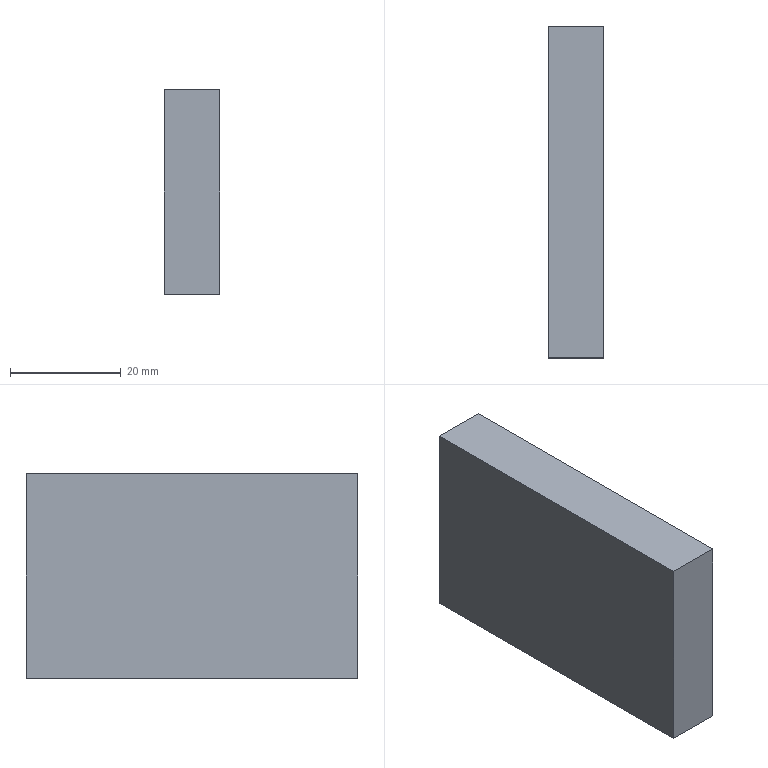Part | NX | features DATUM_CSYS 2, EXTRUDE 1, SKETCH 1 | 1 solid | 6 faces | box 10 x 60 x 37 mm | volume 22200 mm3 | plane 6
STEP:
#1=CARTESIAN_POINT('',(0.,-30.,18.5));
#2=VERTEX_POINT('',#1);
#3=CARTESIAN_POINT('',(0.,-30.,-18.5));
#4=VERTEX_POINT('',#3);
#5=CARTESIAN_POINT('',(0.,-30.,18.5));
#6=DIRECTION('',(0.,0.,-1.));
#7=VECTOR('',#6,1000.);
#8=LINE('',#5,#7);
#9=EDGE_CURVE('',#2,#4,#8,.T.);
#10=ORIENTED_EDGE('',*,*,#9,.T.);
#11=CARTESIAN_POINT('',(10.,-30.,-18.5));
#12=VERTEX_POINT('',#11);
#13=CARTESIAN_POINT('',(10.,-30.,-18.5));
#14=DIRECTION('',(-1.,0.,0.));
#15=VECTOR('',#14,1000.);
#16=LINE('',#13,#15);
#17=EDGE_CURVE('',#12,#4,#16,.T.);
#18=ORIENTED_EDGE('',*,*,#17,.F.);
#19=CARTESIAN_POINT('',(10.,-30.,18.5));
#20=VERTEX_POINT('',#19);
#21=CARTESIAN_POINT('',(10.,-30.,18.5));
#22=DIRECTION('',(0.,0.,-1.));
#23=VECTOR('',#22,1000.);
#24=LINE('',#21,#23);
#25=EDGE_CURVE('',#20,#12,#24,.T.);
#26=ORIENTED_EDGE('',*,*,#25,.F.);
#27=CARTESIAN_POINT('',(10.,-30.,18.5));
#28=DIRECTION('',(-1.,0.,0.));
#29=VECTOR('',#28,1000.);
#30=LINE('',#27,#29);
#31=EDGE_CURVE('',#20,#2,#30,.T.);
#32=ORIENTED_EDGE('',*,*,#31,.T.);
#33=EDGE_LOOP('',(#10,#18,#26,#32));
#34=FACE_BOUND('',#33,.T.);
#35=CARTESIAN_POINT('',(10.,-30.,18.5));
#36=DIRECTION('',(0.,1.,0.));
#37=DIRECTION('',(0.,0.,1.));
#38=AXIS2_PLACEMENT_3D('',#35,#36,#37);
#39=PLANE('',#38);
#40=ADVANCED_FACE('',(#34),#39,.F.);
#41=CARTESIAN_POINT('',(0.,30.,-18.5));
#42=VERTEX_POINT('',#41);
#43=CARTESIAN_POINT('',(0.,-30.,-18.5));
#44=DIRECTION('',(0.,1.,0.));
#45=VECTOR('',#44,1000.);
#46=LINE('',#43,#45);
#47=EDGE_CURVE('',#4,#42,#46,.T.);
#48=ORIENTED_EDGE('',*,*,#47,.T.);
#49=CARTESIAN_POINT('',(10.,30.,-18.5));
#50=VERTEX_POINT('',#49);
#51=CARTESIAN_POINT('',(10.,30.,-18.5));
#52=DIRECTION('',(-1.,0.,0.));
#53=VECTOR('',#52,1000.);
#54=LINE('',#51,#53);
#55=EDGE_CURVE('',#50,#42,#54,.T.);
#56=ORIENTED_EDGE('',*,*,#55,.F.);
#57=CARTESIAN_POINT('',(10.,-30.,-18.5));
#58=DIRECTION('',(0.,1.,0.));
#59=VECTOR('',#58,1000.);
#60=LINE('',#57,#59);
#61=EDGE_CURVE('',#12,#50,#60,.T.);
#62=ORIENTED_EDGE('',*,*,#61,.F.);
#63=ORIENTED_EDGE('',*,*,#17,.T.);
#64=EDGE_LOOP('',(#48,#56,#62,#63));
#65=FACE_BOUND('',#64,.T.);
#66=CARTESIAN_POINT('',(10.,-30.,-18.5));
#67=DIRECTION('',(0.,0.,1.));
#68=DIRECTION('',(1.,0.,0.));
#69=AXIS2_PLACEMENT_3D('',#66,#67,#68);
#70=PLANE('',#69);
#71=ADVANCED_FACE('',(#65),#70,.F.);
#72=CARTESIAN_POINT('',(0.,30.,18.5));
#73=VERTEX_POINT('',#72);
#74=CARTESIAN_POINT('',(0.,30.,-18.5));
#75=DIRECTION('',(0.,0.,1.));
#76=VECTOR('',#75,1000.);
#77=LINE('',#74,#76);
#78=EDGE_CURVE('',#42,#73,#77,.T.);
#79=ORIENTED_EDGE('',*,*,#78,.T.);
#80=CARTESIAN_POINT('',(10.,30.,18.5));
#81=VERTEX_POINT('',#80);
#82=CARTESIAN_POINT('',(10.,30.,18.5));
#83=DIRECTION('',(-1.,0.,0.));
#84=VECTOR('',#83,1000.);
#85=LINE('',#82,#84);
#86=EDGE_CURVE('',#81,#73,#85,.T.);
#87=ORIENTED_EDGE('',*,*,#86,.F.);
#88=CARTESIAN_POINT('',(10.,30.,-18.5));
#89=DIRECTION('',(0.,0.,1.));
#90=VECTOR('',#89,1000.);
#91=LINE('',#88,#90);
#92=EDGE_CURVE('',#50,#81,#91,.T.);
#93=ORIENTED_EDGE('',*,*,#92,.F.);
#94=ORIENTED_EDGE('',*,*,#55,.T.);
#95=EDGE_LOOP('',(#79,#87,#93,#94));
#96=FACE_BOUND('',#95,.T.);
#97=CARTESIAN_POINT('',(10.,30.,-18.5));
#98=DIRECTION('',(0.,-1.,0.));
#99=DIRECTION('',(0.,0.,-1.));
#100=AXIS2_PLACEMENT_3D('',#97,#98,#99);
#101=PLANE('',#100);
#102=ADVANCED_FACE('',(#96),#101,.F.);
#103=CARTESIAN_POINT('',(0.,30.,18.5));
#104=DIRECTION('',(0.,-1.,0.));
#105=VECTOR('',#104,1000.);
#106=LINE('',#103,#105);
#107=EDGE_CURVE('',#73,#2,#106,.T.);
#108=ORIENTED_EDGE('',*,*,#107,.T.);
#109=ORIENTED_EDGE('',*,*,#31,.F.);
#110=CARTESIAN_POINT('',(10.,30.,18.5));
#111=DIRECTION('',(0.,-1.,0.));
#112=VECTOR('',#111,1000.);
#113=LINE('',#110,#112);
#114=EDGE_CURVE('',#81,#20,#113,.T.);
#115=ORIENTED_EDGE('',*,*,#114,.F.);
#116=ORIENTED_EDGE('',*,*,#86,.T.);
#117=EDGE_LOOP('',(#108,#109,#115,#116));
#118=FACE_BOUND('',#117,.T.);
#119=CARTESIAN_POINT('',(10.,30.,18.5));
#120=DIRECTION('',(0.,0.,-1.));
#121=DIRECTION('',(-1.,0.,0.));
#122=AXIS2_PLACEMENT_3D('',#119,#120,#121);
#123=PLANE('',#122);
#124=ADVANCED_FACE('',(#118),#123,.F.);
#125=ORIENTED_EDGE('',*,*,#25,.T.);
#126=ORIENTED_EDGE('',*,*,#61,.T.);
#127=ORIENTED_EDGE('',*,*,#92,.T.);
#128=ORIENTED_EDGE('',*,*,#114,.T.);
#129=EDGE_LOOP('',(#125,#126,#127,#128));
#130=FACE_BOUND('',#129,.T.);
#131=CARTESIAN_POINT('',(10.,0.,0.));
#132=DIRECTION('',(1.,0.,0.));
#133=DIRECTION('',(0.,0.,-1.));
#134=AXIS2_PLACEMENT_3D('',#131,#132,#133);
#135=PLANE('',#134);
#136=ADVANCED_FACE('',(#130),#135,.T.);
#137=ORIENTED_EDGE('',*,*,#9,.F.);
#138=ORIENTED_EDGE('',*,*,#107,.F.);
#139=ORIENTED_EDGE('',*,*,#78,.F.);
#140=ORIENTED_EDGE('',*,*,#47,.F.);
#141=EDGE_LOOP('',(#137,#138,#139,#140));
#142=FACE_BOUND('',#141,.T.);
#143=CARTESIAN_POINT('',(0.,0.,0.));
#144=DIRECTION('',(1.,0.,0.));
#145=DIRECTION('',(0.,0.,-1.));
#146=AXIS2_PLACEMENT_3D('',#143,#144,#145);
#147=PLANE('',#146);
#148=ADVANCED_FACE('',(#142),#147,.F.);
#149=CLOSED_SHELL('',(#40,#71,#102,#124,#136,#148));
#150=MANIFOLD_SOLID_BREP('',#149);
#151=(LENGTH_UNIT()NAMED_UNIT(*)SI_UNIT(.MILLI.,.METRE.));
#152=UNCERTAINTY_MEASURE_WITH_UNIT(LENGTH_MEASURE(0.00001),#151,'','');
#153=(NAMED_UNIT(*)PLANE_ANGLE_UNIT()SI_UNIT($,.RADIAN.));
#154=(NAMED_UNIT(*)SI_UNIT($,.STERADIAN.)SOLID_ANGLE_UNIT());
#155=(GEOMETRIC_REPRESENTATION_CONTEXT(3)GLOBAL_UNCERTAINTY_ASSIGNED_CONTEXT((#152))GLOBAL_UNIT_ASSIGNED_CONTEXT((#151,#153,#154))REPRESENTATION_CONTEXT('',''));
#156=ADVANCED_BREP_SHAPE_REPRESENTATION('',(#150),#155);